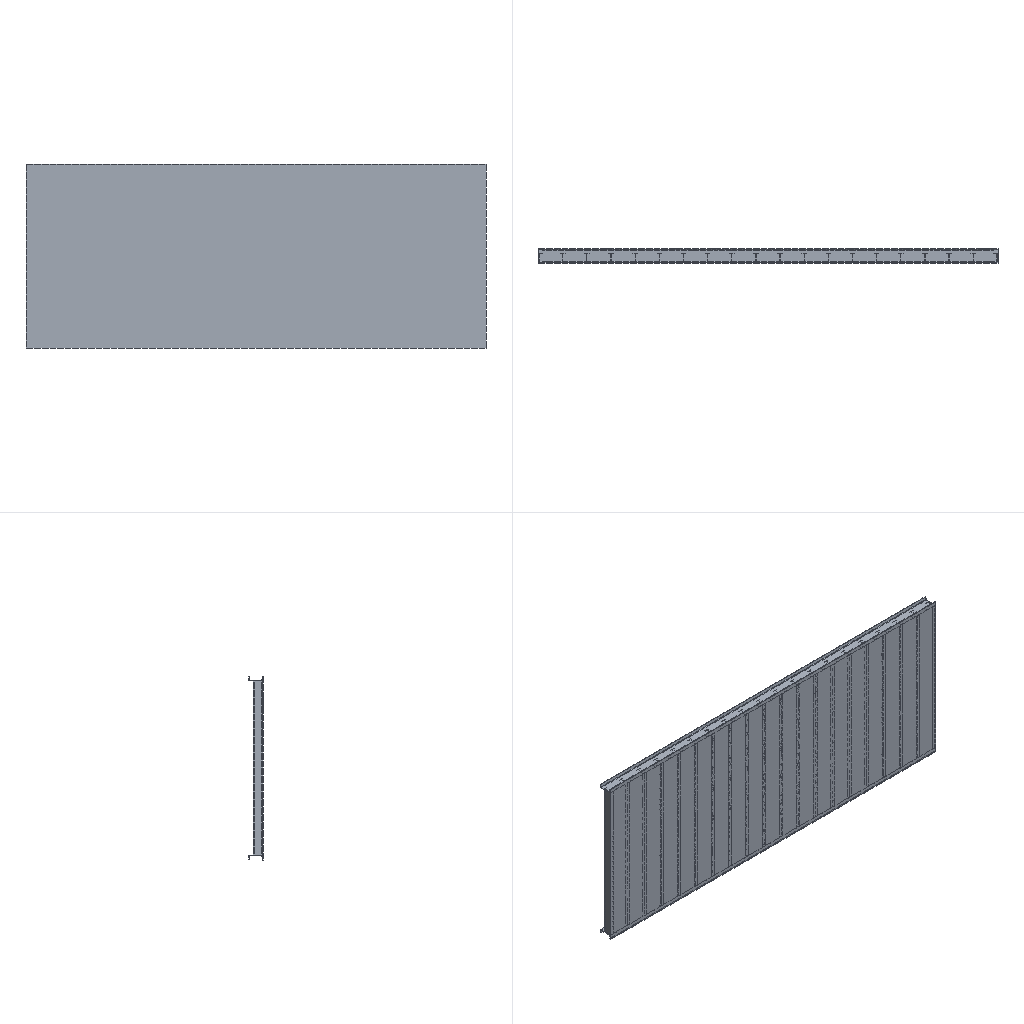Simulation study
Ansys APDL input file, long lists of numbers shortened:
/batch
/config,noeldb,1     ! force off writing results to database
*get,_wallstrt,active,,time,wall
! ANSYS input file written by Workbench version 2022 R1
! File used for geometry attach: F:\ansys（分析文件汇总)\结构件有限元分析qqww\1040mutai_asm.STEP
/title,11--____ (B5)
! ****** Begin Custom Load Command Snippet ******
/COM, ACT Extensions:
/COM,     LSDYNA, 2021.1
/COM,
! ****** End   Custom Load Command Snippet ******
*DIM,_wb_ProjectScratch_dir,string,248
_wb_ProjectScratch_dir(1) = 'F:\ansys（分析文件汇总)\结构件有限元分析qqww\_ProjectScratch\Scr9A7C\'
*DIM,_wb_SolverFiles_dir,string,248
_wb_SolverFiles_dir(1) = 'F:\ansys（分析文件汇总)\结构件有限元分析qqww\11_files\dp0\SYS\MECH\'
*DIM,_wb_userfiles_dir,string,248
_wb_userfiles_dir(1) = 'F:\ansys（分析文件汇总)\结构件有限元分析qqww\11_files\user_files\'
/com,--- Data in consistent NMM units. See Solving Units in the help system for more information.
/units,MPA
/nopr
/wb,file,start              !  signify a WB generated input file
/prep7
! Turn off shape checking because checks already performed inside WB mesher.
! See help system for more information.
SHPP,OFF,,NOWARN
/nolist
etcon,set             ! allow ANSYS to choose best KEYOP's for 180x elements, resets any applicable keyopt to MAPDL defaults
/com,*********** Nodes for the whole assembly ***********
nblock,3,,218006
(1i9,3e20.9e3)
        1    -5.500000000E+02     0.000000000E+00    -5.500000000E+02
! (198187 more lines like these left out)
-1
/wb,elem,start            !  set before creation of elements
/com,*********** Elements for Body 1 "1040MUTAI-1|1040MUTAI-1[1]" ***********
et,1,187
eblock,19,solid,,24901
(19i9)
        1        1        1        1        0        0        0        0       10        0        1      144     6330     7934     7194     9903    47517     9905     9904
! (49801 more lines like these left out)
-1
/com,*********** Elements for Body 2 "1040MUTAI-2|1040MUTAI-2[1]" ***********
et,2,187
eblock,19,solid,,3615
(19i9)
        2        2        2        2        0        0        0        0       10        0    54918   109741   109779   109778   109817   112233   112395   112232   112235
! (7229 more lines like these left out)
-1
/com,*********** Elements for Body 3 "1040MUTAI-2|1040MUTAI-2[1][2]" ***********
et,3,187
eblock,19,solid,,3615
(19i9)
        3        3        3        3        0        0        0        0       10        0    33228    68533    68571    68570    68609    71025    71187    71024    71027
! (7229 more lines like these left out)
-1
/com,*********** Elements for Body 4 "1040MUTAI-2|1040MUTAI-2[1][3]" ***********
et,4,187
eblock,19,solid,,3615
(19i9)
        4        4        4        4        0        0        0        0       10        0    62148   123477   123515   123514   123553   125969   126131   125968   125971
! (7229 more lines like these left out)
-1
/com,*********** Elements for Body 5 "1040MUTAI-2|1040MUTAI-2[1][4]" ***********
et,5,187
eblock,19,solid,,3615
(19i9)
        5        5        5        5        0        0        0        0       10        0    78356   158233   158271   158270   158309   160725   160887   160724   160727
! (7229 more lines like these left out)
-1
! (18 more sections like these left out)
/wb,elem,end               !  done creating elements
/com,*********** Send User Defined Coordinate System(s) ***********
csys,0
toffst,273.15,  ! Temperature offset from absolute zero
/com,*********** Set Reference Temperature ***********
tref,22.
/wb,mat,start              !  starting to send materials
/com,*********** Send Materials ***********
Temperature = 'TEMP' ! Temperature
MP,DENS,1,7.85e-09,	! tonne mm^-3
MP,ALPX,1,1.2e-05,	! C^-1
MP,C,1,434000000,	! mm^2 s^-2 C^-1
MP,KXX,1,60.5,	! tonne mm s^-3 C^-1
MP,RSVX,1,0.00017,	! ohm mm
MP,EX,1,200000,	! tonne s^-2 mm^-1
MP,NUXY,1,0.3,
MP,MURX,1,10000,
Temperature = 'TEMP' ! Temperature
MP,DENS,2,7.85e-09,	! tonne mm^-3
MP,ALPX,2,1.2e-05,	! C^-1
MP,C,2,434000000,	! mm^2 s^-2 C^-1
MP,KXX,2,60.5,	! tonne mm s^-3 C^-1
MP,RSVX,2,0.00017,	! ohm mm
MP,EX,2,200000,	! tonne s^-2 mm^-1
MP,NUXY,2,0.3,
MP,MURX,2,10000,
Temperature = 'TEMP' ! Temperature
MP,DENS,3,7.85e-09,	! tonne mm^-3
MP,ALPX,3,1.2e-05,	! C^-1
MP,C,3,434000000,	! mm^2 s^-2 C^-1
MP,KXX,3,60.5,	! tonne mm s^-3 C^-1
MP,RSVX,3,0.00017,	! ohm mm
MP,EX,3,200000,	! tonne s^-2 mm^-1
MP,NUXY,3,0.3,
MP,MURX,3,10000,
Temperature = 'TEMP' ! Temperature
MP,DENS,4,7.85e-09,	! tonne mm^-3
MP,ALPX,4,1.2e-05,	! C^-1
MP,C,4,434000000,	! mm^2 s^-2 C^-1
MP,KXX,4,60.5,	! tonne mm s^-3 C^-1
MP,RSVX,4,0.00017,	! ohm mm
MP,EX,4,200000,	! tonne s^-2 mm^-1
MP,NUXY,4,0.3,
MP,MURX,4,10000,
Temperature = 'TEMP' ! Temperature
MP,DENS,5,7.85e-09,	! tonne mm^-3
MP,ALPX,5,1.2e-05,	! C^-1
MP,C,5,434000000,	! mm^2 s^-2 C^-1
MP,KXX,5,60.5,	! tonne mm s^-3 C^-1
MP,RSVX,5,0.00017,	! ohm mm
MP,EX,5,200000,	! tonne s^-2 mm^-1
MP,NUXY,5,0.3,
MP,MURX,5,10000,
Temperature = 'TEMP' ! Temperature
MP,DENS,6,7.85e-09,	! tonne mm^-3
MP,ALPX,6,1.2e-05,	! C^-1
MP,C,6,434000000,	! mm^2 s^-2 C^-1
MP,KXX,6,60.5,	! tonne mm s^-3 C^-1
MP,RSVX,6,0.00017,	! ohm mm
MP,EX,6,200000,	! tonne s^-2 mm^-1
MP,NUXY,6,0.3,
MP,MURX,6,10000,
Temperature = 'TEMP' ! Temperature
MP,DENS,7,7.85e-09,	! tonne mm^-3
MP,ALPX,7,1.2e-05,	! C^-1
MP,C,7,434000000,	! mm^2 s^-2 C^-1
MP,KXX,7,60.5,	! tonne mm s^-3 C^-1
MP,RSVX,7,0.00017,	! ohm mm
MP,EX,7,200000,	! tonne s^-2 mm^-1
MP,NUXY,7,0.3,
MP,MURX,7,10000,
Temperature = 'TEMP' ! Temperature
MP,DENS,8,7.85e-09,	! tonne mm^-3
MP,ALPX,8,1.2e-05,	! C^-1
MP,C,8,434000000,	! mm^2 s^-2 C^-1
MP,KXX,8,60.5,	! tonne mm s^-3 C^-1
MP,RSVX,8,0.00017,	! ohm mm
MP,EX,8,200000,	! tonne s^-2 mm^-1
MP,NUXY,8,0.3,
MP,MURX,8,10000,
Temperature = 'TEMP' ! Temperature
MP,DENS,9,7.85e-09,	! tonne mm^-3
MP,ALPX,9,1.2e-05,	! C^-1
MP,C,9,434000000,	! mm^2 s^-2 C^-1
MP,KXX,9,60.5,	! tonne mm s^-3 C^-1
MP,RSVX,9,0.00017,	! ohm mm
MP,EX,9,200000,	! tonne s^-2 mm^-1
! (128 more lines like these left out)
/wb,mat,end                !  done sending materials
!************************* Model Summary ********************
!1040MUTAI-1|1040MUTAI-1[1],	Q235,	matid,	1
!1040MUTAI-2|1040MUTAI-2[1],	Q235,	matid,	2
!1040MUTAI-2|1040MUTAI-2[1][2],	Q235,	matid,	3
!1040MUTAI-2|1040MUTAI-2[1][3],	Q235,	matid,	4
!1040MUTAI-2|1040MUTAI-2[1][4],	Q235,	matid,	5
!1040MUTAI-2|1040MUTAI-2[1][5],	Q235,	matid,	6
!1040MUTAI-2|1040MUTAI-2[1][6],	Q235,	matid,	7
!1040MUTAI-2|1040MUTAI-2[1][7],	Q235,	matid,	8
!1040MUTAI-2|1040MUTAI-2[1][8],	Q235,	matid,	9
!1040MUTAI-2|1040MUTAI-2[1][9],	Q235,	matid,	10
!1040MUTAI-2|1040MUTAI-2[1][10],	Q235,	matid,	11
!1040MUTAI-2|1040MUTAI-2[1][11],	Q235,	matid,	12
!1040MUTAI-2|1040MUTAI-2[1][12],	Q235,	matid,	13
!1040MUTAI-2|1040MUTAI-2[1][13],	Q235,	matid,	14
!1040MUTAI-2|1040MUTAI-2[1][14],	Q235,	matid,	15
!1040MUTAI-2|1040MUTAI-2[1][15],	Q235,	matid,	16
!1040MUTAI-2|1040MUTAI-2[1][16],	Q235,	matid,	17
!1040MUTAI-2|1040MUTAI-2[1][17],	Q235,	matid,	18
!1040MUTAI-2|1040MUTAI-2[1][18],	Q235,	matid,	19
!CAOGANG_300_85_7|CAOGANG_300_85_7[1],	Q235,	matid,	20
!CAOGANG_300_85_7|CAOGANG_300_85_7[1][2],	Q235,	matid,	21
!CAOGANG_200_75_9|CAOGANG_200_75_9[1],	Q235,	matid,	22
!CAOGANG_200_75_9|CAOGANG_200_75_9[1][2],	Q235,	matid,	23
!************************* End Model Summary ********************
! get the diagonal of the bounding box. Needed later for other things
*get,_xmin,node,,mnloc,x
*get,_ymin,node,,mnloc,y
*get,_zmin,node,,mnloc,z
*get,_xmax,node,,mxloc,x
*get,_ymax,node,,mxloc,y
*get,_zmax,node,,mxloc,z
_ASMDIAG=(_xmax-_xmin)*(_xmax-_xmin)+(_ymax-_ymin)*(_ymax-_ymin)+(_zmax-_zmin)*(_zmax-_zmin)
_ASMDIAG=SQRT(_ASMDIAG)
/wb,contact,start          !  starting to send contact
/com,*********** Create Contact "接触区域" ***********
/com,            Real Constant Set For Above Contact Is 25 & 24
*set,tid,25
*set,cid,24
r,tid
r,cid
et,tid,170
et,cid,174
eblock,10,,,243
(15i9)
   159544       25       25       25        0     7272     8023     7797     7797    49569    50235     7797    49568
! (242 more lines like these left out)
-1
eblock,10,,,243
(15i9)
   159787       24       24       24        0     7272     8023     7797     7797    49569    50235     7797    49568
! (242 more lines like these left out)
-1
eblock,10,,,152
(15i9)
   160030       24       25       24        0   110601   109710   110624   110624   111990   111991   110624   116393
! (151 more lines like these left out)
-1
eblock,10,,,152
(15i9)
   160182       25       24       25        0   110601   109710   110624   110624   111990   111991   110624   116393
! (151 more lines like these left out)
-1
keyo,cid,8,2               ! auto create asymmetric contact (from Program Controlled setting)
keyo,cid,10,0              ! adjust contact stiffness each NR iteration (from Program Controlled setting)
keyo,cid,12,5              ! bonded always
keyo,cid,18,1              ! small sliding turned on by application
keyo,cid,2,0               ! augmented Lagrange (from Program Controlled setting)
keyo,cid,4,0               ! on Gauss point (from Program Controlled setting)
keyo,cid,9,1               ! ignore initial gaps/penetration
keyo,cid,7,0               ! No Prediction
rmod,tid,3,10.      ! FKN
rmod,tid,5,0.       ! ICONT
rmod,tid,6,0.       ! PINB
rmod,tid,10,0.      ! CNOF
rmod,tid,12,0.      ! FKT
rmod,tid,36,92      ! WB DSID
rmod,cid,3,10.      ! FKN
rmod,cid,5,0.       ! ICONT
rmod,cid,6,0.       ! PINB
rmod,cid,10,0.      ! CNOF
rmod,cid,12,0.      ! FKT
rmod,cid,36,92      ! WB DSID
/com,*********** Create Contact "接触区域 2" ***********
/com,            Real Constant Set For Above Contact Is 27 & 26
*set,tid,27
*set,cid,26
r,tid
r,cid
et,tid,170
et,cid,174
eblock,10,,,253
(15i9)
   160334       27       27       27        0     6984     7473     8441     8441    49095    49885     8441    49096
! (252 more lines like these left out)
-1
eblock,10,,,253
(15i9)
   160587       26       26       26        0     6984     7473     8441     8441    49095    49885     8441    49096
! (252 more lines like these left out)
-1
eblock,10,,,152
(15i9)
   160840       26       27       26        0    69393    68502    69416    69416    70782    70783    69416    75185
! (151 more lines like these left out)
-1
eblock,10,,,152
(15i9)
   160992       27       26       27        0    69393    68502    69416    69416    70782    70783    69416    75185
! (151 more lines like these left out)
-1
keyo,cid,8,2               ! auto create asymmetric contact (from Program Controlled setting)
keyo,cid,10,0              ! adjust contact stiffness each NR iteration (from Program Controlled setting)
keyo,cid,12,5              ! bonded always
keyo,cid,18,1              ! small sliding turned on by application
keyo,cid,2,0               ! augmented Lagrange (from Program Controlled setting)
keyo,cid,4,0               ! on Gauss point (from Program Controlled setting)
keyo,cid,9,1               ! ignore initial gaps/penetration
keyo,cid,7,0               ! No Prediction
rmod,tid,3,10.      ! FKN
rmod,tid,5,0.       ! ICONT
rmod,tid,6,0.       ! PINB
rmod,tid,10,0.      ! CNOF
rmod,tid,12,0.      ! FKT
rmod,tid,36,95      ! WB DSID
rmod,cid,3,10.      ! FKN
rmod,cid,5,0.       ! ICONT
rmod,cid,6,0.       ! PINB
rmod,cid,10,0.      ! CNOF
rmod,cid,12,0.      ! FKT
rmod,cid,36,95      ! WB DSID
/com,*********** Create Contact "接触区域 3" ***********
/com,            Real Constant Set For Above Contact Is 29 & 28
*set,tid,29
*set,cid,28
r,tid
r,cid
et,tid,170
et,cid,174
eblock,10,,,241
(15i9)
   161144       29       29       29        0     5050     5837     7570     7570    41701    45791     7570    41706
! (240 more lines like these left out)
-1
eblock,10,,,241
(15i9)
   161385       28       28       28        0     5050     5837     7570     7570    41701    45791     7570    41706
! (240 more lines like these left out)
-1
eblock,10,,,152
(15i9)
   161626       28       29       28        0   124337   123446   124360   124360   125726   125727   124360   130129
! (151 more lines like these left out)
-1
eblock,10,,,152
(15i9)
   161778       29       28       29        0   124337   123446   124360   124360   125726   125727   124360   130129
! (151 more lines like these left out)
-1
keyo,cid,8,2               ! auto create asymmetric contact (from Program Controlled setting)
keyo,cid,10,0              ! adjust contact stiffness each NR iteration (from Program Controlled setting)
keyo,cid,12,5              ! bonded always
keyo,cid,18,1              ! small sliding turned on by application
keyo,cid,2,0               ! augmented Lagrange (from Program Controlled setting)
keyo,cid,4,0               ! on Gauss point (from Program Controlled setting)
keyo,cid,9,1               ! ignore initial gaps/penetration
keyo,cid,7,0               ! No Prediction
rmod,tid,3,10.      ! FKN
rmod,tid,5,0.       ! ICONT
rmod,tid,6,0.       ! PINB
rmod,tid,10,0.      ! CNOF
rmod,tid,12,0.      ! FKT
rmod,tid,36,98      ! WB DSID
rmod,cid,3,10.      ! FKN
rmod,cid,5,0.       ! ICONT
rmod,cid,6,0.       ! PINB
rmod,cid,10,0.      ! CNOF
rmod,cid,12,0.      ! FKT
rmod,cid,36,98      ! WB DSID
/com,*********** Create Contact "接触区域 4" ***********
/com,            Real Constant Set For Above Contact Is 31 & 30
*set,tid,31
*set,cid,30
r,tid
r,cid
et,tid,170
et,cid,174
eblock,10,,,239
(15i9)
   161930       31       31       31        0     6218     7273     7629     7629    47167    49571     7629    47168
! (238 more lines like these left out)
-1
eblock,10,,,239
(15i9)
   162169       30       30       30        0     6218     7273     7629     7629    47167    49571     7629    47168
! (238 more lines like these left out)
-1
eblock,10,,,152
(15i9)
   162408       30       31       30        0   159093   158202   159116   159116   160482   160483   159116   164885
! (151 more lines like these left out)
-1
eblock,10,,,152
(15i9)
   162560       31       30       31        0   159093   158202   159116   159116   160482   160483   159116   164885
! (151 more lines like these left out)
-1
keyo,cid,8,2               ! auto create asymmetric contact (from Program Controlled setting)
keyo,cid,10,0              ! adjust contact stiffness each NR iteration (from Program Controlled setting)
keyo,cid,12,5              ! bonded always
keyo,cid,18,1              ! small sliding turned on by application
keyo,cid,2,0               ! augmented Lagrange (from Program Controlled setting)
keyo,cid,4,0               ! on Gauss point (from Program Controlled setting)
keyo,cid,9,1               ! ignore initial gaps/penetration
keyo,cid,7,0               ! No Prediction
rmod,tid,3,10.      ! FKN
rmod,tid,5,0.       ! ICONT
rmod,tid,6,0.       ! PINB
rmod,tid,10,0.      ! CNOF
rmod,tid,12,0.      ! FKT
rmod,tid,36,101     ! WB DSID
rmod,cid,3,10.      ! FKN
rmod,cid,5,0.       ! ICONT
rmod,cid,6,0.       ! PINB
rmod,cid,10,0.      ! CNOF
rmod,cid,12,0.      ! FKT
rmod,cid,36,101     ! WB DSID
/com,*********** Create Contact "接触区域 5" ***********
/com,            Real Constant Set For Above Contact Is 33 & 32
*set,tid,33
*set,cid,32
r,tid
r,cid
et,tid,170
et,cid,174
eblock,10,,,275
(15i9)
   162712       33       33       33        0     4762     6417     6197     6197    39897    47099     6197    39895
! (274 more lines like these left out)
-1
eblock,10,,,275
(15i9)
   162987       32       32       32        0     4762     6417     6197     6197    39897    47099     6197    39895
! (274 more lines like these left out)
-1
eblock,10,,,152
(15i9)
   163262       32       33       32        0   138073   137182   138096   138096   139462   139463   138096   143865
! (151 more lines like these left out)
-1
eblock,10,,,152
(15i9)
   163414       33       32       33        0   138073   137182   138096   138096   139462   139463   138096   143865
! (151 more lines like these left out)
-1
keyo,cid,8,2               ! auto create asymmetric contact (from Program Controlled setting)
keyo,cid,10,0              ! adjust contact stiffness each NR iteration (from Program Controlled setting)
keyo,cid,12,5              ! bonded always
keyo,cid,18,1              ! small sliding turned on by application
keyo,cid,2,0               ! augmented Lagrange (from Program Controlled setting)
keyo,cid,4,0               ! on Gauss point (from Program Controlled setting)
keyo,cid,9,1               ! ignore initial gaps/penetration
keyo,cid,7,0               ! No Prediction
rmod,tid,3,10.      ! FKN
rmod,tid,5,0.       ! ICONT
rmod,tid,6,0.       ! PINB
rmod,tid,10,0.      ! CNOF
rmod,tid,12,0.      ! FKT
rmod,tid,36,104     ! WB DSID
rmod,cid,3,10.      ! FKN
rmod,cid,5,0.       ! ICONT
rmod,cid,6,0.       ! PINB
rmod,cid,10,0.      ! CNOF
rmod,cid,12,0.      ! FKT
rmod,cid,36,104     ! WB DSID
! (57 more sections like these left out)
/wb,contact,end            !  done creating contacts
/golist
/wb,load,start             !  starting to send loads
/com,*********** Fixed Supports ***********
CMBLOCK,_FIXEDSU,NODE,     1206
(8i10)
     50672     50673     51380     51381     51382     51383     51384     51385
! (150 more lines like these left out)
cmsel,s,_FIXEDSU
d,all,all
nsel,all
/com,*********** Define Force Using Surface Effect Elements ***********
local,12,0,0.,0.,0.,0.,0.,0.
csys,0
et,148,154
eblock,10,,,918
(15i9)
   180546      148      148      148       12      322      323     2044     2044    11545    11558     2044    11548
! (917 more lines like these left out)
-1
esel,s,type,,148
keyop,148,2,1                ! Apply load in local coordinate system
keyop,148,7,1                ! Use original area so load is constant in large deformation
esel,all
/com,*********** Define Force Using Surface Effect Elements ***********
local,13,0,0.,0.,0.,0.,0.,0.
csys,0
et,149,154
eblock,10,,,216
(15i9)
   181464      149      149      149       13       46     4547     4580     4580     9002    38612     4580     9003
! (215 more lines like these left out)
-1
esel,s,type,,149
keyop,149,2,1                ! Apply load in local coordinate system
keyop,149,7,1                ! Use original area so load is constant in large deformation
esel,all
/gst,on,on
fini
*get,_numnode,node,0,count
*get,_numelem,elem,0,count
*get, _MAXELEMNUM, elem, 0, NUM, MAX
*get, _MAXNODENUM, node, 0, NUM, MAX
*get, _MAXELEMTYPE, etyp, 0, NUM, MAX
*get, _MAXREALCONST, real, 0, NUM, MAX
/go
/wb,load,end               !  done creating loads
/com,--- Number of total nodes = %_numnode%
/com,--- Number of contact elements = 22136
/com,--- Number of spring elements = 0
/com,--- Number of bearing elements = 0
/com,--- Number of solid elements = 99495
/com,--- Number of condensed parts = 0
/com,--- Number of total elements = %_numelem%
*get,_wallbsol,active,,time,wall
/com,****************************************************************************
/com,*************************    SOLUTION       ********************************
/com,****************************************************************************
/solu
antype,0                   ! static analysis
_thickRatio=0.087   ! Ratio of thick parts in the model
eqsl,sparse,,,,,1
cntr,print,1               ! print out contact info and also make no initial contact an error
dmpoption,emat,no             ! Don't combine emat file for DANSYS
dmpoption,esav,no             ! Don't combine esav file for DANSYS
nldiag,cont,iter           ! print out contact info each equilibrium iteration
rescontrol,,none                 ! Do not keep any restart files
/com,****************************************************
/com,******************* SOLVE FOR LS 1 OF 1 ****************
esel,s,type,,148
nsle
sfe,all,1,pres,1,0.
sfe,all,2,pres,1,6.55725419664067e-002
sfe,all,3,pres,1,0.
esel,s,type,,149
nsle
sfe,all,1,pres,1,0.
sfe,all,2,pres,1,0.2083
sfe,all,3,pres,1,0.
nsel,all
esel,all
acel,0.,0.,9806.65
/nopr
/gopr
nsub,1,1,1
time,1.
outres,erase
outres,all,none
outres,nsol,all,
outres,rsol,all
outres,eangl,all
outres,etmp,all
outres,veng,all
outres,strs,all,
outres,epel,all,
outres,eppl,all,
outres,cont,all,
! *********** WB SOLVE COMMAND ***********
! check interactive state
*get,ANSINTER_,active,,int
*if,ANSINTER_,ne,0,then
/eof
*endif
solve
/com *************** Write FE CONNECTORS *********
CEWRITE,file,ce,,INTE
/com,****************************************************
/com,*************** FINISHED SOLVE FOR LS 1 *************
*get,_wallasol,active,,time,wall
/nopr
*get,_numnode,node,0,count
*get,_numelem,elem,0,count
*get, _MAXELEMNUM, elem, 0, NUM, MAX
*get, _MAXNODENUM, node, 0, NUM, MAX,,,INTERNAL
*get, _MAXELEMTYPE, etyp, 0, NUM, MAX
*get, _MAXREALCONST, real, 0, NUM, MAX
/gopr
/post1
xmlo,ENCODING,ISO-8859-1
xmlo,parm
/xml,parm,xml
fini
/gopr
*get,_walldone,active,,time,wall
_preptime=(_wallbsol-_wallstrt)*3600
_solvtime=(_wallasol-_wallbsol)*3600
_posttime=(_walldone-_wallasol)*3600
_totaltim=(_walldone-_wallstrt)*3600
*get,_dlbratio,active,0,solu,dlbr
*get,_combtime,active,0,solu,comb
*get,_ssmode,active,0,solu,ssmm
*get,_ndofs,active,0,solu,ndof
*get,_sol_end_time,active,0,set,time
*if,_sol_end_time,eq,1.,then
/fclean				!clean distributed files
*endif
/com,--- Total number of nodes = %_numnode%
/com,--- Total number of elements = %_numelem%
/com,--- Element load balance ratio = %_dlbratio%
/com,--- Time to combine distributed files = %_combtime%
/com,--- Sparse memory mode = %_ssmode%
/com,--- Number of DOF = %_ndofs%
/wb,file,end               ! done with WB generated input